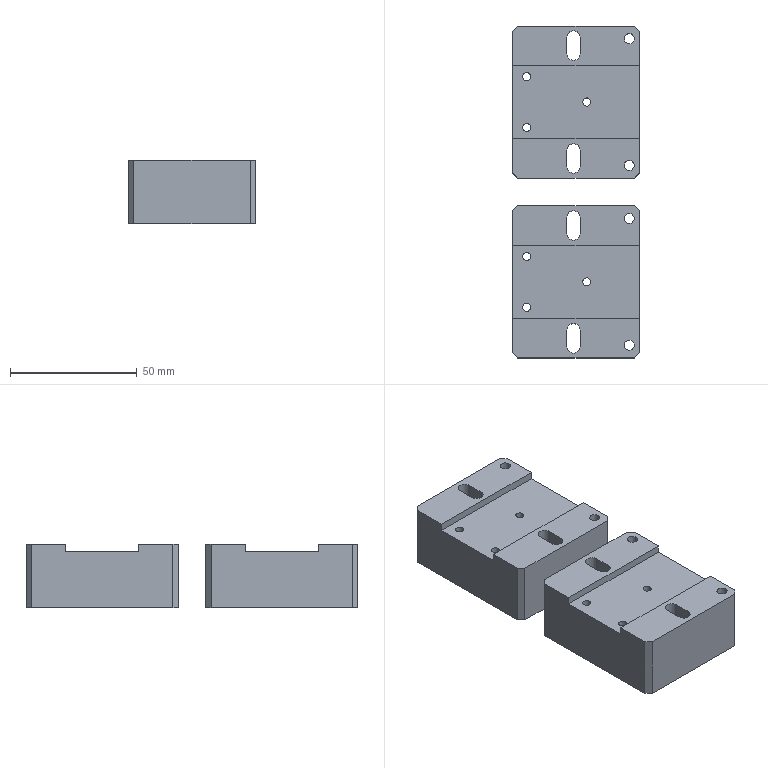Part | 2 solids | 66 faces | box 50 x 131 x 25 mm | volume 132224 mm3 | plane 42 | cylinder 24 | commonest cylinder face diameters 5.2 x8 3.2 x6 6 x6 4 x4